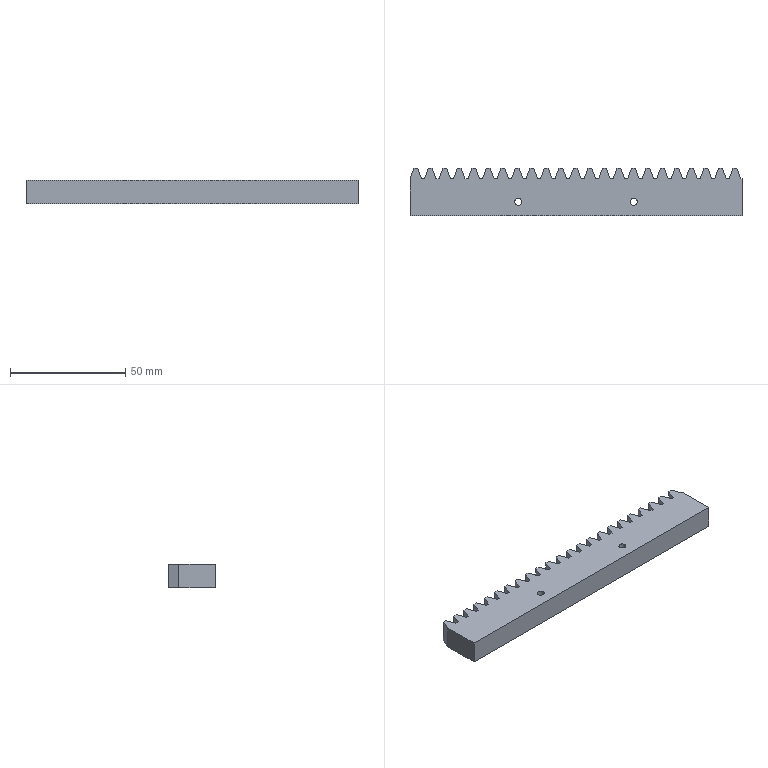Part | SolidWorks | features BaseBody 1 | 1 solid | 101 faces | box 143.769 x 20.5 x 10 mm | volume 26301 mm3 | plane 97 | cylinder 4 | commonest cylinder face diameters 3 x4